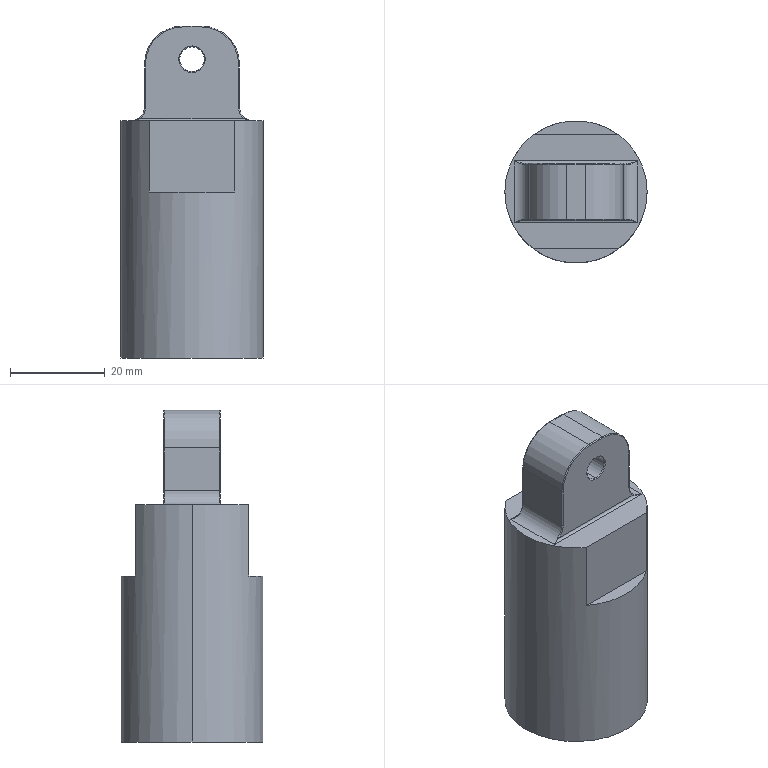Part | NX | features BREP 1 | 1 solid | 47 faces | box 30 x 30 x 70 mm | volume 29940 mm3 | cylinder 18 | plane 11 | torus 8 | cone 6 | spline 4 | commonest cylinder face diameters 0.4 x6 1 x2 5.2 x2 6 x2 16 x2 18.5 x2
STEP:
#1=CARTESIAN_POINT('',(0.,-5.8,65.6));
#2=VERTEX_POINT('',#1);
#3=CARTESIAN_POINT('',(0.,-5.8,60.4));
#4=VERTEX_POINT('',#3);
#5=CARTESIAN_POINT('',(0.,-5.8,63.));
#6=DIRECTION('',(0.,-1.,0.));
#7=DIRECTION('',(0.,0.,1.));
#8=AXIS2_PLACEMENT_3D('',#5,#6,#7);
#9=CIRCLE('',#8,2.6);
#10=EDGE_CURVE('',#2,#4,#9,.T.);
#11=ORIENTED_EDGE('',*,*,#10,.F.);
#12=CARTESIAN_POINT('',(0.,-6.,65.8));
#13=VERTEX_POINT('',#12);
#14=CARTESIAN_POINT('',(0.,-6.,65.8));
#15=DIRECTION('',(0.,-0.7071,0.7071));
#16=VECTOR('',#15,1000.);
#17=LINE('',#14,#16);
#18=EDGE_CURVE('',#2,#13,#17,.T.);
#19=ORIENTED_EDGE('',*,*,#18,.T.);
#20=CARTESIAN_POINT('',(0.,-6.,60.2));
#21=VERTEX_POINT('',#20);
#22=CARTESIAN_POINT('',(0.,-6.,63.));
#23=DIRECTION('',(0.,1.,0.));
#24=DIRECTION('',(-1.,0.,0.));
#25=AXIS2_PLACEMENT_3D('',#22,#23,#24);
#26=CIRCLE('',#25,2.8);
#27=EDGE_CURVE('',#21,#13,#26,.T.);
#28=ORIENTED_EDGE('',*,*,#27,.F.);
#29=CARTESIAN_POINT('',(0.,-6.,60.2));
#30=DIRECTION('',(0.,-0.7071,-0.7071));
#31=VECTOR('',#30,1000.);
#32=LINE('',#29,#31);
#33=EDGE_CURVE('',#4,#21,#32,.T.);
#34=ORIENTED_EDGE('',*,*,#33,.F.);
#35=EDGE_LOOP('',(#11,#19,#28,#34));
#36=FACE_BOUND('',#35,.T.);
#37=CARTESIAN_POINT('',(0.,-6.,63.));
#38=DIRECTION('',(0.,-1.,0.));
#39=DIRECTION('',(0.,0.,-1.));
#40=AXIS2_PLACEMENT_3D('',#37,#38,#39);
#41=CONICAL_SURFACE('',#40,2.8,0.7854);
#42=ADVANCED_FACE('',(#36),#41,.F.);
#43=CARTESIAN_POINT('',(0.,5.8,60.4));
#44=VERTEX_POINT('',#43);
#45=CARTESIAN_POINT('',(0.,5.8,65.6));
#46=VERTEX_POINT('',#45);
#47=CARTESIAN_POINT('',(0.,5.8,63.));
#48=DIRECTION('',(0.,1.,0.));
#49=DIRECTION('',(0.,0.,-1.));
#50=AXIS2_PLACEMENT_3D('',#47,#48,#49);
#51=CIRCLE('',#50,2.6);
#52=EDGE_CURVE('',#44,#46,#51,.T.);
#53=ORIENTED_EDGE('',*,*,#52,.F.);
#54=CARTESIAN_POINT('',(0.,6.,60.2));
#55=VERTEX_POINT('',#54);
#56=CARTESIAN_POINT('',(0.,5.8,60.4));
#57=DIRECTION('',(0.,0.7071,-0.7071));
#58=VECTOR('',#57,1000.);
#59=LINE('',#56,#58);
#60=EDGE_CURVE('',#55,#44,#59,.F.);
#61=ORIENTED_EDGE('',*,*,#60,.F.);
#62=CARTESIAN_POINT('',(0.,6.,65.8));
#63=VERTEX_POINT('',#62);
#64=CARTESIAN_POINT('',(0.,6.,63.));
#65=DIRECTION('',(0.,-1.,0.));
#66=DIRECTION('',(1.,0.,0.));
#67=AXIS2_PLACEMENT_3D('',#64,#65,#66);
#68=CIRCLE('',#67,2.8);
#69=EDGE_CURVE('',#63,#55,#68,.T.);
#70=ORIENTED_EDGE('',*,*,#69,.F.);
#71=CARTESIAN_POINT('',(0.,5.8,65.6));
#72=DIRECTION('',(0.,0.7071,0.7071));
#73=VECTOR('',#72,1000.);
#74=LINE('',#71,#73);
#75=EDGE_CURVE('',#63,#46,#74,.F.);
#76=ORIENTED_EDGE('',*,*,#75,.T.);
#77=EDGE_LOOP('',(#53,#61,#70,#76));
#78=FACE_BOUND('',#77,.T.);
#79=CARTESIAN_POINT('',(0.,5.8,63.));
#80=DIRECTION('',(0.,1.,0.));
#81=DIRECTION('',(0.,0.,1.));
#82=AXIS2_PLACEMENT_3D('',#79,#80,#81);
#83=CONICAL_SURFACE('',#82,2.6,0.7854);
#84=ADVANCED_FACE('',(#78),#83,.F.);
#85=ORIENTED_EDGE('',*,*,#10,.T.);
#86=CARTESIAN_POINT('',(0.,6.,60.4));
#87=DIRECTION('',(0.,1.,0.));
#88=VECTOR('',#87,1000.);
#89=LINE('',#86,#88);
#90=EDGE_CURVE('',#44,#4,#89,.F.);
#91=ORIENTED_EDGE('',*,*,#90,.F.);
#92=ORIENTED_EDGE('',*,*,#52,.T.);
#93=CARTESIAN_POINT('',(0.,6.,65.6));
#94=DIRECTION('',(0.,1.,0.));
#95=VECTOR('',#94,1000.);
#96=LINE('',#93,#95);
#97=EDGE_CURVE('',#46,#2,#96,.F.);
#98=ORIENTED_EDGE('',*,*,#97,.T.);
#99=EDGE_LOOP('',(#85,#91,#92,#98));
#100=FACE_BOUND('',#99,.T.);
#101=CARTESIAN_POINT('',(0.,6.,63.));
#102=DIRECTION('',(0.,1.,0.));
#103=DIRECTION('',(0.,0.,1.));
#104=AXIS2_PLACEMENT_3D('',#101,#102,#103);
#105=CYLINDRICAL_SURFACE('',#104,2.6);
#106=ADVANCED_FACE('',(#100),#105,.F.);
#107=CARTESIAN_POINT('',(9.25,0.,30.));
#108=VERTEX_POINT('',#107);
#109=CARTESIAN_POINT('',(-9.25,0.,30.));
#110=VERTEX_POINT('',#109);
#111=CARTESIAN_POINT('',(0.,0.,30.));
#112=DIRECTION('',(0.,0.,-1.));
#113=DIRECTION('',(-1.,0.,0.));
#114=AXIS2_PLACEMENT_3D('',#111,#112,#113);
#115=CIRCLE('',#114,9.25);
#116=EDGE_CURVE('',#108,#110,#115,.T.);
#117=ORIENTED_EDGE('',*,*,#116,.F.);
#118=CARTESIAN_POINT('',(9.25,0.,0.));
#119=VERTEX_POINT('',#118);
#120=CARTESIAN_POINT('',(9.25,0.,0.));
#121=DIRECTION('',(0.,0.,-1.));
#122=VECTOR('',#121,1000.);
#123=LINE('',#120,#122);
#124=EDGE_CURVE('',#108,#119,#123,.T.);
#125=ORIENTED_EDGE('',*,*,#124,.T.);
#126=CARTESIAN_POINT('',(-9.25,0.,0.));
#127=VERTEX_POINT('',#126);
#128=CARTESIAN_POINT('',(0.,0.,0.));
#129=DIRECTION('',(0.,0.,-1.));
#130=DIRECTION('',(-1.,0.,0.));
#131=AXIS2_PLACEMENT_3D('',#128,#129,#130);
#132=CIRCLE('',#131,9.25);
#133=EDGE_CURVE('',#119,#127,#132,.T.);
#134=ORIENTED_EDGE('',*,*,#133,.T.);
#135=CARTESIAN_POINT('',(-9.25,0.,0.));
#136=DIRECTION('',(0.,0.,-1.));
#137=VECTOR('',#136,1000.);
#138=LINE('',#135,#137);
#139=EDGE_CURVE('',#110,#127,#138,.T.);
#140=ORIENTED_EDGE('',*,*,#139,.F.);
#141=EDGE_LOOP('',(#117,#125,#134,#140));
#142=FACE_BOUND('',#141,.T.);
#143=CARTESIAN_POINT('',(0.,0.,0.));
#144=DIRECTION('',(0.,0.,-1.));
#145=DIRECTION('',(-1.,0.,0.));
#146=AXIS2_PLACEMENT_3D('',#143,#144,#145);
#147=CYLINDRICAL_SURFACE('',#146,9.25);
#148=ADVANCED_FACE('',(#142),#147,.F.);
#149=CARTESIAN_POINT('',(0.,0.,35.558));
#150=VERTEX_POINT('',#149);
#151=CARTESIAN_POINT('',(-9.25,0.,30.));
#152=DIRECTION('',(-0.8572,0.,-0.515));
#153=VECTOR('',#152,1000.);
#154=LINE('',#151,#153);
#155=EDGE_CURVE('',#150,#110,#154,.T.);
#156=ORIENTED_EDGE('',*,*,#155,.F.);
#157=CARTESIAN_POINT('',(9.25,0.,30.));
#158=DIRECTION('',(0.8572,0.,-0.515));
#159=VECTOR('',#158,1000.);
#160=LINE('',#157,#159);
#161=EDGE_CURVE('',#150,#108,#160,.T.);
#162=ORIENTED_EDGE('',*,*,#161,.T.);
#163=ORIENTED_EDGE('',*,*,#116,.T.);
#164=EDGE_LOOP('',(#156,#162,#163));
#165=FACE_BOUND('',#164,.T.);
#166=CARTESIAN_POINT('',(0.,0.,30.));
#167=DIRECTION('',(0.,0.,-1.));
#168=DIRECTION('',(-1.,0.,0.));
#169=AXIS2_PLACEMENT_3D('',#166,#167,#168);
#170=CONICAL_SURFACE('',#169,9.25,1.03);
#171=ADVANCED_FACE('',(#165),#170,.F.);
#172=CARTESIAN_POINT('',(15.,0.,50.));
#173=VERTEX_POINT('',#172);
#174=CARTESIAN_POINT('',(9.,12.,50.));
#175=VERTEX_POINT('',#174);
#176=CARTESIAN_POINT('',(0.,0.,50.));
#177=DIRECTION('',(0.,0.,1.));
#178=DIRECTION('',(1.,0.,0.));
#179=AXIS2_PLACEMENT_3D('',#176,#177,#178);
#180=CIRCLE('',#179,15.);
#181=EDGE_CURVE('',#173,#175,#180,.T.);
#182=ORIENTED_EDGE('',*,*,#181,.F.);
#183=CARTESIAN_POINT('',(15.,0.,0.));
#184=VERTEX_POINT('',#183);
#185=CARTESIAN_POINT('',(15.,0.,50.));
#186=DIRECTION('',(0.,0.,-1.));
#187=VECTOR('',#186,1000.);
#188=LINE('',#185,#187);
#189=EDGE_CURVE('',#173,#184,#188,.T.);
#190=ORIENTED_EDGE('',*,*,#189,.T.);
#191=CARTESIAN_POINT('',(-15.,0.,0.));
#192=VERTEX_POINT('',#191);
#193=CARTESIAN_POINT('',(0.,0.,0.));
#194=DIRECTION('',(0.,0.,1.));
#195=DIRECTION('',(1.,0.,0.));
#196=AXIS2_PLACEMENT_3D('',#193,#194,#195);
#197=CIRCLE('',#196,15.);
#198=EDGE_CURVE('',#184,#192,#197,.T.);
#199=ORIENTED_EDGE('',*,*,#198,.T.);
#200=CARTESIAN_POINT('',(-15.,0.,50.));
#201=VERTEX_POINT('',#200);
#202=CARTESIAN_POINT('',(-15.,0.,50.));
#203=DIRECTION('',(0.,0.,-1.));
#204=VECTOR('',#203,1000.);
#205=LINE('',#202,#204);
#206=EDGE_CURVE('',#201,#192,#205,.T.);
#207=ORIENTED_EDGE('',*,*,#206,.F.);
#208=CARTESIAN_POINT('',(-9.,12.,50.));
#209=VERTEX_POINT('',#208);
#210=CARTESIAN_POINT('',(0.,0.,50.));
#211=DIRECTION('',(0.,0.,1.));
#212=DIRECTION('',(1.,0.,0.));
#213=AXIS2_PLACEMENT_3D('',#210,#211,#212);
#214=CIRCLE('',#213,15.);
#215=EDGE_CURVE('',#209,#201,#214,.T.);
#216=ORIENTED_EDGE('',*,*,#215,.F.);
#217=CARTESIAN_POINT('',(-9.,12.,35.));
#218=VERTEX_POINT('',#217);
#219=CARTESIAN_POINT('',(-9.,12.,50.));
#220=DIRECTION('',(0.,0.,1.));
#221=VECTOR('',#220,1000.);
#222=LINE('',#219,#221);
#223=EDGE_CURVE('',#218,#209,#222,.T.);
#224=ORIENTED_EDGE('',*,*,#223,.F.);
#225=CARTESIAN_POINT('',(9.,12.,35.));
#226=VERTEX_POINT('',#225);
#227=CARTESIAN_POINT('',(0.,0.,35.));
#228=DIRECTION('',(0.,0.,1.));
#229=DIRECTION('',(1.,0.,0.));
#230=AXIS2_PLACEMENT_3D('',#227,#228,#229);
#231=CIRCLE('',#230,15.);
#232=EDGE_CURVE('',#226,#218,#231,.T.);
#233=ORIENTED_EDGE('',*,*,#232,.F.);
#234=CARTESIAN_POINT('',(9.,12.,50.));
#235=DIRECTION('',(0.,0.,-1.));
#236=VECTOR('',#235,1000.);
#237=LINE('',#234,#236);
#238=EDGE_CURVE('',#175,#226,#237,.T.);
#239=ORIENTED_EDGE('',*,*,#238,.F.);
#240=EDGE_LOOP('',(#182,#190,#199,#207,#216,#224,#233,#239));
#241=FACE_BOUND('',#240,.T.);
#242=CARTESIAN_POINT('',(0.,0.,50.));
#243=DIRECTION('',(0.,0.,-1.));
#244=DIRECTION('',(-1.,0.,0.));
#245=AXIS2_PLACEMENT_3D('',#242,#243,#244);
#246=CYLINDRICAL_SURFACE('',#245,15.);
#247=ADVANCED_FACE('',(#241),#246,.T.);
#248=ORIENTED_EDGE('',*,*,#189,.F.);
#249=CARTESIAN_POINT('',(9.,-12.,50.));
#250=VERTEX_POINT('',#249);
#251=CARTESIAN_POINT('',(0.,0.,50.));
#252=DIRECTION('',(0.,0.,1.));
#253=DIRECTION('',(1.,0.,0.));
#254=AXIS2_PLACEMENT_3D('',#251,#252,#253);
#255=CIRCLE('',#254,15.);
#256=EDGE_CURVE('',#250,#173,#255,.T.);
#257=ORIENTED_EDGE('',*,*,#256,.F.);
#258=CARTESIAN_POINT('',(9.,-12.,35.));
#259=VERTEX_POINT('',#258);
#260=CARTESIAN_POINT('',(9.,-12.,50.));
#261=DIRECTION('',(0.,0.,1.));
#262=VECTOR('',#261,1000.);
#263=LINE('',#260,#262);
#264=EDGE_CURVE('',#259,#250,#263,.T.);
#265=ORIENTED_EDGE('',*,*,#264,.F.);
#266=CARTESIAN_POINT('',(-9.,-12.,35.));
#267=VERTEX_POINT('',#266);
#268=CARTESIAN_POINT('',(0.,0.,35.));
#269=DIRECTION('',(0.,0.,1.));
#270=DIRECTION('',(1.,0.,0.));
#271=AXIS2_PLACEMENT_3D('',#268,#269,#270);
#272=CIRCLE('',#271,15.);
#273=EDGE_CURVE('',#267,#259,#272,.T.);
#274=ORIENTED_EDGE('',*,*,#273,.F.);
#275=CARTESIAN_POINT('',(-9.,-12.,50.));
#276=VERTEX_POINT('',#275);
#277=CARTESIAN_POINT('',(-9.,-12.,50.));
#278=DIRECTION('',(0.,0.,-1.));
#279=VECTOR('',#278,1000.);
#280=LINE('',#277,#279);
#281=EDGE_CURVE('',#276,#267,#280,.T.);
#282=ORIENTED_EDGE('',*,*,#281,.F.);
#283=CARTESIAN_POINT('',(0.,0.,50.));
#284=DIRECTION('',(0.,0.,1.));
#285=DIRECTION('',(1.,0.,0.));
#286=AXIS2_PLACEMENT_3D('',#283,#284,#285);
#287=CIRCLE('',#286,15.);
#288=EDGE_CURVE('',#201,#276,#287,.T.);
#289=ORIENTED_EDGE('',*,*,#288,.F.);
#290=ORIENTED_EDGE('',*,*,#206,.T.);
#291=CARTESIAN_POINT('',(0.,0.,0.));
#292=DIRECTION('',(0.,0.,1.));
#293=DIRECTION('',(1.,0.,0.));
#294=AXIS2_PLACEMENT_3D('',#291,#292,#293);
#295=CIRCLE('',#294,15.);
#296=EDGE_CURVE('',#192,#184,#295,.T.);
#297=ORIENTED_EDGE('',*,*,#296,.T.);
#298=EDGE_LOOP('',(#248,#257,#265,#274,#282,#289,#290,#297));
#299=FACE_BOUND('',#298,.T.);
#300=CARTESIAN_POINT('',(0.,0.,50.));
#301=DIRECTION('',(0.,0.,-1.));
#302=DIRECTION('',(-1.,0.,0.));
#303=AXIS2_PLACEMENT_3D('',#300,#301,#302);
#304=CYLINDRICAL_SURFACE('',#303,15.);
#305=ADVANCED_FACE('',(#299),#304,.T.);
#306=ORIENTED_EDGE('',*,*,#256,.T.);
#307=ORIENTED_EDGE('',*,*,#181,.T.);
#308=CARTESIAN_POINT('',(0.,12.,50.));
#309=DIRECTION('',(-1.,0.,0.));
#310=VECTOR('',#309,1000.);
#311=LINE('',#308,#310);
#312=EDGE_CURVE('',#175,#209,#311,.T.);
#313=ORIENTED_EDGE('',*,*,#312,.T.);
#314=ORIENTED_EDGE('',*,*,#215,.T.);
#315=ORIENTED_EDGE('',*,*,#288,.T.);
#316=CARTESIAN_POINT('',(0.,-12.,50.));
#317=DIRECTION('',(1.,0.,0.));
#318=VECTOR('',#317,1000.);
#319=LINE('',#316,#318);
#320=EDGE_CURVE('',#276,#250,#319,.T.);
#321=ORIENTED_EDGE('',*,*,#320,.T.);
#322=EDGE_LOOP('',(#306,#307,#313,#314,#315,#321));
#323=FACE_BOUND('',#322,.T.);
#324=CARTESIAN_POINT('',(13.,6.5,50.));
#325=VERTEX_POINT('',#324);
#326=CARTESIAN_POINT('',(13.,-6.5,50.));
#327=VERTEX_POINT('',#326);
#328=CARTESIAN_POINT('',(13.,0.,50.));
#329=DIRECTION('',(0.,-1.,0.));
#330=VECTOR('',#329,1000.);
#331=LINE('',#328,#330);
#332=EDGE_CURVE('',#325,#327,#331,.T.);
#333=ORIENTED_EDGE('',*,*,#332,.T.);
#334=CARTESIAN_POINT('',(-13.,-6.5,50.));
#335=VERTEX_POINT('',#334);
#336=CARTESIAN_POINT('',(0.,-6.5,50.));
#337=DIRECTION('',(-1.,0.,0.));
#338=VECTOR('',#337,1000.);
#339=LINE('',#336,#338);
#340=EDGE_CURVE('',#327,#335,#339,.T.);
#341=ORIENTED_EDGE('',*,*,#340,.T.);
#342=CARTESIAN_POINT('',(-13.,6.5,50.));
#343=VERTEX_POINT('',#342);
#344=CARTESIAN_POINT('',(-13.,0.,50.));
#345=DIRECTION('',(0.,1.,0.));
#346=VECTOR('',#345,1000.);
#347=LINE('',#344,#346);
#348=EDGE_CURVE('',#335,#343,#347,.T.);
#349=ORIENTED_EDGE('',*,*,#348,.T.);
#350=CARTESIAN_POINT('',(0.,6.5,50.));
#351=DIRECTION('',(1.,0.,0.));
#352=VECTOR('',#351,1000.);
#353=LINE('',#350,#352);
#354=EDGE_CURVE('',#343,#325,#353,.T.);
#355=ORIENTED_EDGE('',*,*,#354,.T.);
#356=EDGE_LOOP('',(#333,#341,#349,#355));
#357=FACE_BOUND('',#356,.T.);
#358=CARTESIAN_POINT('',(0.,0.,50.));
#359=DIRECTION('',(0.,0.,1.));
#360=DIRECTION('',(1.,0.,0.));
#361=AXIS2_PLACEMENT_3D('',#358,#359,#360);
#362=PLANE('',#361);
#363=ADVANCED_FACE('',(#323,#357),#362,.T.);
#364=ORIENTED_EDGE('',*,*,#296,.F.);
#365=ORIENTED_EDGE('',*,*,#198,.F.);
#366=EDGE_LOOP('',(#364,#365));
#367=FACE_BOUND('',#366,.T.);
#368=CARTESIAN_POINT('',(0.,0.,0.));
#369=DIRECTION('',(0.,0.,-1.));
#370=DIRECTION('',(-1.,0.,0.));
#371=AXIS2_PLACEMENT_3D('',#368,#369,#370);
#372=CIRCLE('',#371,9.25);
#373=EDGE_CURVE('',#127,#119,#372,.T.);
#374=ORIENTED_EDGE('',*,*,#373,.F.);
#375=ORIENTED_EDGE('',*,*,#133,.F.);
#376=EDGE_LOOP('',(#374,#375));
#377=FACE_BOUND('',#376,.T.);
#378=CARTESIAN_POINT('',(0.,0.,0.));
#379=DIRECTION('',(0.,0.,1.));
#380=DIRECTION('',(1.,0.,0.));
#381=AXIS2_PLACEMENT_3D('',#378,#379,#380);
#382=PLANE('',#381);
#383=ADVANCED_FACE('',(#367,#377),#382,.F.);
#384=ORIENTED_EDGE('',*,*,#161,.F.);
#385=ORIENTED_EDGE('',*,*,#155,.T.);
#386=CARTESIAN_POINT('',(0.,0.,30.));
#387=DIRECTION('',(0.,0.,-1.));
#388=DIRECTION('',(-1.,0.,0.));
#389=AXIS2_PLACEMENT_3D('',#386,#387,#388);
#390=CIRCLE('',#389,9.25);
#391=EDGE_CURVE('',#110,#108,#390,.T.);
#392=ORIENTED_EDGE('',*,*,#391,.T.);
#393=EDGE_LOOP('',(#384,#385,#392));
#394=FACE_BOUND('',#393,.T.);
#395=CARTESIAN_POINT('',(0.,0.,30.));
#396=DIRECTION('',(0.,0.,-1.));
#397=DIRECTION('',(-1.,0.,0.));
#398=AXIS2_PLACEMENT_3D('',#395,#396,#397);
#399=CONICAL_SURFACE('',#398,9.25,1.03);
#400=ADVANCED_FACE('',(#394),#399,.F.);
#401=ORIENTED_EDGE('',*,*,#124,.F.);
#402=ORIENTED_EDGE('',*,*,#391,.F.);
#403=ORIENTED_EDGE('',*,*,#139,.T.);
#404=ORIENTED_EDGE('',*,*,#373,.T.);
#405=EDGE_LOOP('',(#401,#402,#403,#404));
#406=FACE_BOUND('',#405,.T.);
#407=CARTESIAN_POINT('',(0.,0.,0.));
#408=DIRECTION('',(0.,0.,-1.));
#409=DIRECTION('',(-1.,0.,0.));
#410=AXIS2_PLACEMENT_3D('',#407,#408,#409);
#411=CYLINDRICAL_SURFACE('',#410,9.25);
#412=ADVANCED_FACE('',(#406),#411,.F.);
#413=CARTESIAN_POINT('',(-10.,5.8,53.));
#414=VERTEX_POINT('',#413);
#415=CARTESIAN_POINT('',(-10.,-5.8,53.));
#416=VERTEX_POINT('',#415);
#417=CARTESIAN_POINT('',(-10.,-6.,53.));
#418=DIRECTION('',(0.,-1.,0.));
#419=VECTOR('',#418,1000.);
#420=LINE('',#417,#419);
#421=EDGE_CURVE('',#414,#416,#420,.T.);
#422=ORIENTED_EDGE('',*,*,#421,.T.);
#423=CARTESIAN_POINT('',(-10.,-5.8,62.));
#424=VERTEX_POINT('',#423);
#425=CARTESIAN_POINT('',(-10.,-5.8,70.));
#426=DIRECTION('',(0.,0.,1.));
#427=VECTOR('',#426,1000.);
#428=LINE('',#425,#427);
#429=EDGE_CURVE('',#416,#424,#428,.T.);
#430=ORIENTED_EDGE('',*,*,#429,.T.);
#431=CARTESIAN_POINT('',(-10.,5.8,62.));
#432=VERTEX_POINT('',#431);
#433=CARTESIAN_POINT('',(-10.,6.,62.));
#434=DIRECTION('',(0.,1.,0.));
#435=VECTOR('',#434,1000.);
#436=LINE('',#433,#435);
#437=EDGE_CURVE('',#424,#432,#436,.T.);
#438=ORIENTED_EDGE('',*,*,#437,.T.);
#439=CARTESIAN_POINT('',(-10.,5.8,70.));
#440=DIRECTION('',(0.,0.,-1.));
#441=VECTOR('',#440,1000.);
#442=LINE('',#439,#441);
#443=EDGE_CURVE('',#432,#414,#442,.T.);
#444=ORIENTED_EDGE('',*,*,#443,.T.);
#445=EDGE_LOOP('',(#422,#430,#438,#444));
#446=FACE_BOUND('',#445,.T.);
#447=CARTESIAN_POINT('',(-10.,-6.,70.));
#448=DIRECTION('',(1.,0.,0.));
#449=DIRECTION('',(0.,1.,0.));
#450=AXIS2_PLACEMENT_3D('',#447,#448,#449);
#451=PLANE('',#450);
#452=ADVANCED_FACE('',(#446),#451,.F.);
#453=CARTESIAN_POINT('',(-11.003,-6.,50.5));
#454=VERTEX_POINT('',#453);
#455=CARTESIAN_POINT('',(11.003,-6.,50.5));
#456=VERTEX_POINT('',#455);
#457=CARTESIAN_POINT('',(10.,-6.,50.5));
#458=DIRECTION('',(1.,0.,0.));
#459=VECTOR('',#458,1000.);
#460=LINE('',#457,#459);
#461=EDGE_CURVE('',#454,#456,#460,.T.);
#462=ORIENTED_EDGE('',*,*,#461,.T.);
#463=CARTESIAN_POINT('',(9.8,-6.,53.));
#464=VERTEX_POINT('',#463);
#465=CARTESIAN_POINT('',(13.,-6.,53.));
#466=DIRECTION('',(0.,1.,0.));
#467=DIRECTION('',(-1.,0.,0.));
#468=AXIS2_PLACEMENT_3D('',#465,#466,#467);
#469=CIRCLE('',#468,3.2);
#470=EDGE_CURVE('',#456,#464,#469,.T.);
#471=ORIENTED_EDGE('',*,*,#470,.T.);
#472=CARTESIAN_POINT('',(9.8,-6.,62.));
#473=VERTEX_POINT('',#472);
#474=CARTESIAN_POINT('',(9.8,-6.,70.));
#475=DIRECTION('',(0.,0.,1.));
#476=VECTOR('',#475,1000.);
#477=LINE('',#474,#476);
#478=EDGE_CURVE('',#464,#473,#477,.T.);
#479=ORIENTED_EDGE('',*,*,#478,.T.);
#480=CARTESIAN_POINT('',(2.,-6.,69.8));
#481=VERTEX_POINT('',#480);
#482=CARTESIAN_POINT('',(2.,-6.,62.));
#483=DIRECTION('',(0.,-1.,0.));
#484=DIRECTION('',(-1.,0.,0.));
#485=AXIS2_PLACEMENT_3D('',#482,#483,#484);
#486=CIRCLE('',#485,7.8);
#487=EDGE_CURVE('',#473,#481,#486,.T.);
#488=ORIENTED_EDGE('',*,*,#487,.T.);
#489=CARTESIAN_POINT('',(-2.,-6.,69.8));
#490=VERTEX_POINT('',#489);
#491=CARTESIAN_POINT('',(-2.,-6.,69.8));
#492=DIRECTION('',(-1.,0.,0.));
#493=VECTOR('',#492,1000.);
#494=LINE('',#491,#493);
#495=EDGE_CURVE('',#481,#490,#494,.T.);
#496=ORIENTED_EDGE('',*,*,#495,.T.);
#497=CARTESIAN_POINT('',(-9.8,-6.,62.));
#498=VERTEX_POINT('',#497);
#499=CARTESIAN_POINT('',(-2.,-6.,62.));
#500=DIRECTION('',(0.,-1.,0.));
#501=DIRECTION('',(-1.,0.,0.));
#502=AXIS2_PLACEMENT_3D('',#499,#500,#501);
#503=CIRCLE('',#502,7.8);
#504=EDGE_CURVE('',#490,#498,#503,.T.);
#505=ORIENTED_EDGE('',*,*,#504,.T.);
#506=CARTESIAN_POINT('',(-9.8,-6.,53.));
#507=VERTEX_POINT('',#506);
#508=CARTESIAN_POINT('',(-9.8,-6.,70.));
#509=DIRECTION('',(0.,0.,-1.));
#510=VECTOR('',#509,1000.);
#511=LINE('',#508,#510);
#512=EDGE_CURVE('',#498,#507,#511,.T.);
#513=ORIENTED_EDGE('',*,*,#512,.T.);
#514=CARTESIAN_POINT('',(-13.,-6.,53.));
#515=DIRECTION('',(0.,1.,0.));
#516=DIRECTION('',(-1.,0.,0.));
#517=AXIS2_PLACEMENT_3D('',#514,#515,#516);
#518=CIRCLE('',#517,3.2);
#519=EDGE_CURVE('',#507,#454,#518,.T.);
#520=ORIENTED_EDGE('',*,*,#519,.T.);
#521=EDGE_LOOP('',(#462,#471,#479,#488,#496,#505,#513,#520));
#522=FACE_BOUND('',#521,.T.);
#523=ORIENTED_EDGE('',*,*,#27,.T.);
#524=CARTESIAN_POINT('',(0.,-6.,63.));
#525=DIRECTION('',(0.,1.,0.));
#526=DIRECTION('',(-1.,0.,0.));
#527=AXIS2_PLACEMENT_3D('',#524,#525,#526);
#528=CIRCLE('',#527,2.8);
#529=EDGE_CURVE('',#13,#21,#528,.T.);
#530=ORIENTED_EDGE('',*,*,#529,.T.);
#531=EDGE_LOOP('',(#523,#530));
#532=FACE_BOUND('',#531,.T.);
#533=CARTESIAN_POINT('',(10.,-6.,70.));
#534=DIRECTION('',(0.,1.,0.));
#535=DIRECTION('',(1.,0.,0.));
#536=AXIS2_PLACEMENT_3D('',#533,#534,#535);
#537=PLANE('',#536);
#538=ADVANCED_FACE('',(#522,#532),#537,.F.);
#539=CARTESIAN_POINT('',(10.,5.8,62.));
#540=VERTEX_POINT('',#539);
#541=CARTESIAN_POINT('',(10.,-5.8,62.));
#542=VERTEX_POINT('',#541);
#543=CARTESIAN_POINT('',(10.,-6.,62.));
#544=DIRECTION('',(0.,-1.,0.));
#545=VECTOR('',#544,1000.);
#546=LINE('',#543,#545);
#547=EDGE_CURVE('',#540,#542,#546,.T.);
#548=ORIENTED_EDGE('',*,*,#547,.T.);
#549=CARTESIAN_POINT('',(10.,-5.8,53.));
#550=VERTEX_POINT('',#549);
#551=CARTESIAN_POINT('',(10.,-5.8,70.));
#552=DIRECTION('',(0.,0.,-1.));
#553=VECTOR('',#552,1000.);
#554=LINE('',#551,#553);
#555=EDGE_CURVE('',#542,#550,#554,.T.);
#556=ORIENTED_EDGE('',*,*,#555,.T.);
#557=CARTESIAN_POINT('',(10.,5.8,53.));
#558=VERTEX_POINT('',#557);
#559=CARTESIAN_POINT('',(10.,-6.,53.));
#560=DIRECTION('',(0.,1.,0.));
#561=VECTOR('',#560,1000.);
#562=LINE('',#559,#561);
#563=EDGE_CURVE('',#550,#558,#562,.T.);
#564=ORIENTED_EDGE('',*,*,#563,.T.);
#565=CARTESIAN_POINT('',(10.,5.8,70.));
#566=DIRECTION('',(0.,0.,1.));
#567=VECTOR('',#566,1000.);
#568=LINE('',#565,#567);
#569=EDGE_CURVE('',#558,#540,#568,.T.);
#570=ORIENTED_EDGE('',*,*,#569,.T.);
#571=EDGE_LOOP('',(#548,#556,#564,#570));
#572=FACE_BOUND('',#571,.T.);
#573=CARTESIAN_POINT('',(10.,-6.,70.));
#574=DIRECTION('',(-1.,0.,0.));
#575=DIRECTION('',(0.,0.,1.));
#576=AXIS2_PLACEMENT_3D('',#573,#574,#575);
#577=PLANE('',#576);
#578=ADVANCED_FACE('',(#572),#577,.F.);
#579=CARTESIAN_POINT('',(9.8,6.,62.));
#580=VERTEX_POINT('',#579);
#581=CARTESIAN_POINT('',(9.8,6.,53.));
#582=VERTEX_POINT('',#581);
#583=CARTESIAN_POINT('',(9.8,6.,70.));
#584=DIRECTION('',(0.,0.,-1.));
#585=VECTOR('',#584,1000.);
#586=LINE('',#583,#585);
#587=EDGE_CURVE('',#580,#582,#586,.T.);
#588=ORIENTED_EDGE('',*,*,#587,.T.);
#589=CARTESIAN_POINT('',(11.003,6.,50.5));
#590=VERTEX_POINT('',#589);
#591=CARTESIAN_POINT('',(13.,6.,53.));
#592=DIRECTION('',(0.,-1.,0.));
#593=DIRECTION('',(1.,0.,0.));
#594=AXIS2_PLACEMENT_3D('',#591,#592,#593);
#595=CIRCLE('',#594,3.2);
#596=EDGE_CURVE('',#582,#590,#595,.T.);
#597=ORIENTED_EDGE('',*,*,#596,.T.);
#598=CARTESIAN_POINT('',(-11.003,6.,50.5));
#599=VERTEX_POINT('',#598);
#600=CARTESIAN_POINT('',(10.,6.,50.5));
#601=DIRECTION('',(-1.,0.,0.));
#602=VECTOR('',#601,1000.);
#603=LINE('',#600,#602);
#604=EDGE_CURVE('',#590,#599,#603,.T.);
#605=ORIENTED_EDGE('',*,*,#604,.T.);
#606=CARTESIAN_POINT('',(-9.8,6.,53.));
#607=VERTEX_POINT('',#606);
#608=CARTESIAN_POINT('',(-13.,6.,53.));
#609=DIRECTION('',(0.,-1.,0.));
#610=DIRECTION('',(1.,0.,0.));
#611=AXIS2_PLACEMENT_3D('',#608,#609,#610);
#612=CIRCLE('',#611,3.2);
#613=EDGE_CURVE('',#599,#607,#612,.T.);
#614=ORIENTED_EDGE('',*,*,#613,.T.);
#615=CARTESIAN_POINT('',(-9.8,6.,62.));
#616=VERTEX_POINT('',#615);
#617=CARTESIAN_POINT('',(-9.8,6.,70.));
#618=DIRECTION('',(0.,0.,1.));
#619=VECTOR('',#618,1000.);
#620=LINE('',#617,#619);
#621=EDGE_CURVE('',#607,#616,#620,.T.);
#622=ORIENTED_EDGE('',*,*,#621,.T.);
#623=CARTESIAN_POINT('',(-2.,6.,69.8));
#624=VERTEX_POINT('',#623);
#625=CARTESIAN_POINT('',(-2.,6.,62.));
#626=DIRECTION('',(0.,1.,0.));
#627=DIRECTION('',(1.,0.,0.));
#628=AXIS2_PLACEMENT_3D('',#625,#626,#627);
#629=CIRCLE('',#628,7.8);
#630=EDGE_CURVE('',#616,#624,#629,.T.);
#631=ORIENTED_EDGE('',*,*,#630,.T.);
#632=CARTESIAN_POINT('',(2.,6.,69.8));
#633=VERTEX_POINT('',#632);
#634=CARTESIAN_POINT('',(2.,6.,69.8));
#635=DIRECTION('',(1.,0.,0.));
#636=VECTOR('',#635,1000.);
#637=LINE('',#634,#636);
#638=EDGE_CURVE('',#624,#633,#637,.T.);
#639=ORIENTED_EDGE('',*,*,#638,.T.);
#640=CARTESIAN_POINT('',(2.,6.,62.));
#641=DIRECTION('',(0.,1.,0.));
#642=DIRECTION('',(1.,0.,0.));
#643=AXIS2_PLACEMENT_3D('',#640,#641,#642);
#644=CIRCLE('',#643,7.8);
#645=EDGE_CURVE('',#633,#580,#644,.T.);
#646=ORIENTED_EDGE('',*,*,#645,.T.);
#647=EDGE_LOOP('',(#588,#597,#605,#614,#622,#631,#639,#646));
#648=FACE_BOUND('',#647,.T.);
#649=ORIENTED_EDGE('',*,*,#69,.T.);
#650=CARTESIAN_POINT('',(0.,6.,63.));
#651=DIRECTION('',(0.,-1.,0.));
#652=DIRECTION('',(1.,0.,0.));
#653=AXIS2_PLACEMENT_3D('',#650,#651,#652);
#654=CIRCLE('',#653,2.8);
#655=EDGE_CURVE('',#55,#63,#654,.T.);
#656=ORIENTED_EDGE('',*,*,#655,.T.);
#657=EDGE_LOOP('',(#649,#656));
#658=FACE_BOUND('',#657,.T.);
#659=CARTESIAN_POINT('',(10.,6.,70.));
#660=DIRECTION('',(0.,-1.,0.));
#661=DIRECTION('',(0.,0.,-1.));
#662=AXIS2_PLACEMENT_3D('',#659,#660,#661);
#663=PLANE('',#662);
#664=ADVANCED_FACE('',(#648,#658),#663,.F.);
#665=CARTESIAN_POINT('',(-2.,5.8,70.));
#666=VERTEX_POINT('',#665);
#667=CARTESIAN_POINT('',(-2.,-5.8,70.));
#668=VERTEX_POINT('',#667);
#669=CARTESIAN_POINT('',(-2.,-6.,70.));
#670=DIRECTION('',(0.,-1.,0.));
#671=VECTOR('',#670,1000.);
#672=LINE('',#669,#671);
#673=EDGE_CURVE('',#666,#668,#672,.T.);
#674=ORIENTED_EDGE('',*,*,#673,.T.);
#675=CARTESIAN_POINT('',(2.,-5.8,70.));
#676=VERTEX_POINT('',#675);
#677=CARTESIAN_POINT('',(2.,-5.8,70.));
#678=DIRECTION('',(1.,0.,0.));
#679=VECTOR('',#678,1000.);
#680=LINE('',#677,#679);
#681=EDGE_CURVE('',#668,#676,#680,.T.);
#682=ORIENTED_EDGE('',*,*,#681,.T.);
#683=CARTESIAN_POINT('',(2.,5.8,70.));
#684=VERTEX_POINT('',#683);
#685=CARTESIAN_POINT('',(2.,6.,70.));
#686=DIRECTION('',(0.,1.,0.));
#687=VECTOR('',#686,1000.);
#688=LINE('',#685,#687);
#689=EDGE_CURVE('',#676,#684,#688,.T.);
#690=ORIENTED_EDGE('',*,*,#689,.T.);
#691=CARTESIAN_POINT('',(-2.,5.8,70.));
#692=DIRECTION('',(-1.,0.,0.));
#693=VECTOR('',#692,1000.);
#694=LINE('',#691,#693);
#695=EDGE_CURVE('',#684,#666,#694,.T.);
#696=ORIENTED_EDGE('',*,*,#695,.T.);
#697=EDGE_LOOP('',(#674,#682,#690,#696));
#698=FACE_BOUND('',#697,.T.);
#699=CARTESIAN_POINT('',(0.,0.,70.));
#700=DIRECTION('',(0.,0.,1.));
#701=DIRECTION('',(1.,0.,0.));
#702=AXIS2_PLACEMENT_3D('',#699,#700,#701);
#703=PLANE('',#702);
#704=ADVANCED_FACE('',(#698),#703,.T.);
#705=ORIENTED_EDGE('',*,*,#90,.T.);
#706=CARTESIAN_POINT('',(0.,-5.8,63.));
#707=DIRECTION('',(0.,-1.,0.));
#708=DIRECTION('',(0.,0.,1.));
#709=AXIS2_PLACEMENT_3D('',#706,#707,#708);
#710=CIRCLE('',#709,2.6);
#711=EDGE_CURVE('',#4,#2,#710,.T.);
#712=ORIENTED_EDGE('',*,*,#711,.T.);
#713=ORIENTED_EDGE('',*,*,#97,.F.);
#714=CARTESIAN_POINT('',(0.,5.8,63.));
#715=DIRECTION('',(0.,1.,0.));
#716=DIRECTION('',(0.,0.,-1.));
#717=AXIS2_PLACEMENT_3D('',#714,#715,#716);
#718=CIRCLE('',#717,2.6);
#719=EDGE_CURVE('',#46,#44,#718,.T.);
#720=ORIENTED_EDGE('',*,*,#719,.T.);
#721=EDGE_LOOP('',(#705,#712,#713,#720));
#722=FACE_BOUND('',#721,.T.);
#723=CARTESIAN_POINT('',(0.,6.,63.));
#724=DIRECTION('',(0.,1.,0.));
#725=DIRECTION('',(0.,0.,1.));
#726=AXIS2_PLACEMENT_3D('',#723,#724,#725);
#727=CYLINDRICAL_SURFACE('',#726,2.6);
#728=ADVANCED_FACE('',(#722),#727,.F.);
#729=CARTESIAN_POINT('',(11.127,-5.8,50.656));
#730=VERTEX_POINT('',#729);
#731=CARTESIAN_POINT('',(13.,-5.8,53.));
#732=DIRECTION('',(0.,-1.,0.));
#733=DIRECTION('',(-1.,0.,0.));
#734=AXIS2_PLACEMENT_3D('',#731,#732,#733);
#735=CIRCLE('',#734,3.);
#736=EDGE_CURVE('',#550,#730,#735,.T.);
#737=ORIENTED_EDGE('',*,*,#736,.T.);
#738=CARTESIAN_POINT('',(11.127,-5.8,50.656));
#739=CARTESIAN_POINT('',(11.24,-5.8,50.567));
#740=CARTESIAN_POINT('',(11.481,-5.832,50.389));
#741=CARTESIAN_POINT('',(11.986,-6.018,50.169));
#742=CARTESIAN_POINT('',(12.246,-6.134,50.093));
#743=CARTESIAN_POINT('',(12.543,-6.273,50.032));
#744=CARTESIAN_POINT('',(12.687,-6.345,50.014));
#745=CARTESIAN_POINT('',(12.89,-6.445,50.));
#746=CARTESIAN_POINT('',(13.,-6.5,50.));
#747=B_SPLINE_CURVE_WITH_KNOTS('',3,(#738,#739,#740,#741,#742,#743,#744,#745,#746),.UNSPECIFIED.,.F.,.F.,(4,1,1,1,1,1,4),(0.,0.25,0.5,0.625,0.75,0.875,1.),.UNSPECIFIED.);
#748=EDGE_CURVE('',#730,#327,#747,.T.);
#749=ORIENTED_EDGE('',*,*,#748,.T.);
#750=ORIENTED_EDGE('',*,*,#332,.F.);
#751=CARTESIAN_POINT('',(11.127,5.8,50.656));
#752=VERTEX_POINT('',#751);
#753=CARTESIAN_POINT('',(13.,6.5,50.));
#754=CARTESIAN_POINT('',(12.889,6.445,50.));
#755=CARTESIAN_POINT('',(12.687,6.345,50.014));
#756=CARTESIAN_POINT('',(12.542,6.273,50.032));
#757=CARTESIAN_POINT('',(12.248,6.134,50.092));
#758=CARTESIAN_POINT('',(11.84,5.955,50.213));
#759=CARTESIAN_POINT('',(11.379,5.8,50.455));
#760=CARTESIAN_POINT('',(11.127,5.8,50.656));
#761=B_SPLINE_CURVE_WITH_KNOTS('',3,(#753,#754,#755,#756,#757,#758,#759,#760),.UNSPECIFIED.,.F.,.F.,(4,1,1,1,1,4),(0.,0.125,0.25,0.375,0.5,1.),.UNSPECIFIED.);
#762=EDGE_CURVE('',#325,#752,#761,.T.);
#763=ORIENTED_EDGE('',*,*,#762,.T.);
#764=CARTESIAN_POINT('',(13.,5.8,53.));
#765=DIRECTION('',(0.,1.,0.));
#766=DIRECTION('',(1.,0.,0.));
#767=AXIS2_PLACEMENT_3D('',#764,#765,#766);
#768=CIRCLE('',#767,3.);
#769=EDGE_CURVE('',#752,#558,#768,.T.);
#770=ORIENTED_EDGE('',*,*,#769,.T.);
#771=ORIENTED_EDGE('',*,*,#563,.F.);
#772=EDGE_LOOP('',(#737,#749,#750,#763,#770,#771));
#773=FACE_BOUND('',#772,.T.);
#774=CARTESIAN_POINT('',(13.,-6.,53.));
#775=DIRECTION('',(0.,1.,0.));
#776=DIRECTION('',(0.,0.,1.));
#777=AXIS2_PLACEMENT_3D('',#774,#775,#776);
#778=CYLINDRICAL_SURFACE('',#777,3.);
#779=ADVANCED_FACE('',(#773),#778,.F.);
#780=ORIENTED_EDGE('',*,*,#348,.F.);
#781=CARTESIAN_POINT('',(-11.127,-5.8,50.656));
#782=VERTEX_POINT('',#781);
#783=CARTESIAN_POINT('',(-13.,-6.5,50.));
#784=CARTESIAN_POINT('',(-12.889,-6.445,50.));
#785=CARTESIAN_POINT('',(-12.687,-6.345,50.014));
#786=CARTESIAN_POINT('',(-12.542,-6.273,50.032));
#787=CARTESIAN_POINT('',(-12.248,-6.134,50.092));
#788=CARTESIAN_POINT('',(-11.84,-5.955,50.213));
#789=CARTESIAN_POINT('',(-11.379,-5.8,50.455));
#790=CARTESIAN_POINT('',(-11.127,-5.8,50.656));
#791=B_SPLINE_CURVE_WITH_KNOTS('',3,(#783,#784,#785,#786,#787,#788,#789,#790),.UNSPECIFIED.,.F.,.F.,(4,1,1,1,1,4),(0.,0.125,0.25,0.375,0.5,1.),.UNSPECIFIED.);
#792=EDGE_CURVE('',#335,#782,#791,.T.);
#793=ORIENTED_EDGE('',*,*,#792,.T.);
#794=CARTESIAN_POINT('',(-13.,-5.8,53.));
#795=DIRECTION('',(0.,-1.,0.));
#796=DIRECTION('',(-1.,0.,0.));
#797=AXIS2_PLACEMENT_3D('',#794,#795,#796);
#798=CIRCLE('',#797,3.);
#799=EDGE_CURVE('',#782,#416,#798,.T.);
#800=ORIENTED_EDGE('',*,*,#799,.T.);
#801=ORIENTED_EDGE('',*,*,#421,.F.);
#802=CARTESIAN_POINT('',(-11.127,5.8,50.656));
#803=VERTEX_POINT('',#802);
#804=CARTESIAN_POINT('',(-13.,5.8,53.));
#805=DIRECTION('',(0.,1.,0.));
#806=DIRECTION('',(1.,0.,0.));
#807=AXIS2_PLACEMENT_3D('',#804,#805,#806);
#808=CIRCLE('',#807,3.);
#809=EDGE_CURVE('',#414,#803,#808,.T.);
#810=ORIENTED_EDGE('',*,*,#809,.T.);
#811=CARTESIAN_POINT('',(-11.127,5.8,50.656));
#812=CARTESIAN_POINT('',(-11.24,5.8,50.567));
#813=CARTESIAN_POINT('',(-11.481,5.832,50.389));
#814=CARTESIAN_POINT('',(-11.986,6.018,50.169));
#815=CARTESIAN_POINT('',(-12.246,6.134,50.093));
#816=CARTESIAN_POINT('',(-12.543,6.273,50.032));
#817=CARTESIAN_POINT('',(-12.687,6.345,50.014));
#818=CARTESIAN_POINT('',(-12.89,6.445,50.));
#819=CARTESIAN_POINT('',(-13.,6.5,50.));
#820=B_SPLINE_CURVE_WITH_KNOTS('',3,(#811,#812,#813,#814,#815,#816,#817,#818,#819),.UNSPECIFIED.,.F.,.F.,(4,1,1,1,1,1,4),(0.,0.25,0.5,0.625,0.75,0.875,1.),.UNSPECIFIED.);
#821=EDGE_CURVE('',#803,#343,#820,.T.);
#822=ORIENTED_EDGE('',*,*,#821,.T.);
#823=EDGE_LOOP('',(#780,#793,#800,#801,#810,#822));
#824=FACE_BOUND('',#823,.T.);
#825=CARTESIAN_POINT('',(-13.,-6.,53.));
#826=DIRECTION('',(0.,-1.,0.));
#827=DIRECTION('',(0.,0.,-1.));
#828=AXIS2_PLACEMENT_3D('',#825,#826,#827);
#829=CYLINDRICAL_SURFACE('',#828,3.);
#830=ADVANCED_FACE('',(#824),#829,.F.);
#831=ORIENTED_EDGE('',*,*,#340,.F.);
#832=CARTESIAN_POINT('',(13.,-6.5,50.));
#833=CARTESIAN_POINT('',(12.769,-6.423,50.));
#834=CARTESIAN_POINT('',(12.475,-6.324,50.025));
#835=CARTESIAN_POINT('',(12.148,-6.225,50.082));
#836=CARTESIAN_POINT('',(12.021,-6.187,50.107));
#837=CARTESIAN_POINT('',(11.67,-6.092,50.202));
#838=CARTESIAN_POINT('',(11.338,-6.023,50.326));
#839=CARTESIAN_POINT('',(11.12,-6.,50.433));
#840=CARTESIAN_POINT('',(11.003,-6.,50.5));
#841=B_SPLINE_CURVE_WITH_KNOTS('',3,(#832,#833,#834,#835,#836,#837,#838,#839,#840),.UNSPECIFIED.,.F.,.F.,(4,1,1,1,1,1,4),(0.,0.25,0.375,0.5,0.625,0.75,1.),.UNSPECIFIED.);
#842=EDGE_CURVE('',#327,#456,#841,.T.);
#843=ORIENTED_EDGE('',*,*,#842,.T.);
#844=ORIENTED_EDGE('',*,*,#461,.F.);
#845=CARTESIAN_POINT('',(-11.003,-6.,50.5));
#846=CARTESIAN_POINT('',(-11.12,-6.,50.433));
#847=CARTESIAN_POINT('',(-11.338,-6.023,50.326));
#848=CARTESIAN_POINT('',(-11.67,-6.092,50.202));
#849=CARTESIAN_POINT('',(-12.021,-6.187,50.107));
#850=CARTESIAN_POINT('',(-12.148,-6.225,50.082));
#851=CARTESIAN_POINT('',(-12.475,-6.324,50.025));
#852=CARTESIAN_POINT('',(-12.768,-6.423,50.));
#853=CARTESIAN_POINT('',(-13.,-6.5,50.));
#854=B_SPLINE_CURVE_WITH_KNOTS('',3,(#845,#846,#847,#848,#849,#850,#851,#852,#853),.UNSPECIFIED.,.F.,.F.,(4,1,1,1,1,1,4),(0.,0.25,0.375,0.5,0.625,0.75,1.),.UNSPECIFIED.);
#855=EDGE_CURVE('',#454,#335,#854,.T.);
#856=ORIENTED_EDGE('',*,*,#855,.T.);
#857=EDGE_LOOP('',(#831,#843,#844,#856));
#858=FACE_BOUND('',#857,.T.);
#859=CARTESIAN_POINT('',(10.,-6.5,50.5));
#860=DIRECTION('',(1.,0.,0.));
#861=DIRECTION('',(0.,1.,0.));
#862=AXIS2_PLACEMENT_3D('',#859,#860,#861);
#863=CYLINDRICAL_SURFACE('',#862,0.5);
#864=ADVANCED_FACE('',(#858),#863,.F.);
#865=ORIENTED_EDGE('',*,*,#604,.F.);
#866=CARTESIAN_POINT('',(11.003,6.,50.5));
#867=CARTESIAN_POINT('',(11.12,6.,50.433));
#868=CARTESIAN_POINT('',(11.338,6.023,50.326));
#869=CARTESIAN_POINT('',(11.67,6.092,50.202));
#870=CARTESIAN_POINT('',(12.021,6.187,50.107));
#871=CARTESIAN_POINT('',(12.148,6.225,50.082));
#872=CARTESIAN_POINT('',(12.475,6.324,50.025));
#873=CARTESIAN_POINT('',(12.768,6.423,50.));
#874=CARTESIAN_POINT('',(13.,6.5,50.));
#875=B_SPLINE_CURVE_WITH_KNOTS('',3,(#866,#867,#868,#869,#870,#871,#872,#873,#874),.UNSPECIFIED.,.F.,.F.,(4,1,1,1,1,1,4),(0.,0.25,0.375,0.5,0.625,0.75,1.),.UNSPECIFIED.);
#876=EDGE_CURVE('',#590,#325,#875,.T.);
#877=ORIENTED_EDGE('',*,*,#876,.T.);
#878=ORIENTED_EDGE('',*,*,#354,.F.);
#879=CARTESIAN_POINT('',(-13.,6.5,50.));
#880=CARTESIAN_POINT('',(-12.769,6.423,50.));
#881=CARTESIAN_POINT('',(-12.475,6.324,50.025));
#882=CARTESIAN_POINT('',(-12.148,6.225,50.082));
#883=CARTESIAN_POINT('',(-12.021,6.187,50.107));
#884=CARTESIAN_POINT('',(-11.67,6.092,50.202));
#885=CARTESIAN_POINT('',(-11.338,6.023,50.326));
#886=CARTESIAN_POINT('',(-11.12,6.,50.433));
#887=CARTESIAN_POINT('',(-11.003,6.,50.5));
#888=B_SPLINE_CURVE_WITH_KNOTS('',3,(#879,#880,#881,#882,#883,#884,#885,#886,#887),.UNSPECIFIED.,.F.,.F.,(4,1,1,1,1,1,4),(0.,0.25,0.375,0.5,0.625,0.75,1.),.UNSPECIFIED.);
#889=EDGE_CURVE('',#343,#599,#888,.T.);
#890=ORIENTED_EDGE('',*,*,#889,.T.);
#891=EDGE_LOOP('',(#865,#877,#878,#890));
#892=FACE_BOUND('',#891,.T.);
#893=CARTESIAN_POINT('',(10.,6.5,50.5));
#894=DIRECTION('',(-1.,0.,0.));
#895=DIRECTION('',(0.,-1.,0.));
#896=AXIS2_PLACEMENT_3D('',#893,#894,#895);
#897=CYLINDRICAL_SURFACE('',#896,0.5);
#898=ADVANCED_FACE('',(#892),#897,.F.);
#899=ORIENTED_EDGE('',*,*,#281,.T.);
#900=CARTESIAN_POINT('',(25.302,-12.,35.));
#901=DIRECTION('',(1.,0.,0.));
#902=VECTOR('',#901,1000.);
#903=LINE('',#900,#902);
#904=EDGE_CURVE('',#267,#259,#903,.T.);
#905=ORIENTED_EDGE('',*,*,#904,.T.);
#906=ORIENTED_EDGE('',*,*,#264,.T.);
#907=ORIENTED_EDGE('',*,*,#320,.F.);
#908=EDGE_LOOP('',(#899,#905,#906,#907));
#909=FACE_BOUND('',#908,.T.);
#910=CARTESIAN_POINT('',(25.302,-12.,35.));
#911=DIRECTION('',(0.,-1.,0.));
#912=DIRECTION('',(0.,0.,-1.));
#913=AXIS2_PLACEMENT_3D('',#910,#911,#912);
#914=PLANE('',#913);
#915=ADVANCED_FACE('',(#909),#914,.T.);
#916=ORIENTED_EDGE('',*,*,#273,.T.);
#917=ORIENTED_EDGE('',*,*,#904,.F.);
#918=EDGE_LOOP('',(#916,#917));
#919=FACE_BOUND('',#918,.T.);
#920=CARTESIAN_POINT('',(0.,0.,35.));
#921=DIRECTION('',(0.,0.,1.));
#922=DIRECTION('',(1.,0.,0.));
#923=AXIS2_PLACEMENT_3D('',#920,#921,#922);
#924=PLANE('',#923);
#925=ADVANCED_FACE('',(#919),#924,.T.);
#926=ORIENTED_EDGE('',*,*,#232,.T.);
#927=CARTESIAN_POINT('',(25.302,12.,35.));
#928=DIRECTION('',(-1.,0.,0.));
#929=VECTOR('',#928,1000.);
#930=LINE('',#927,#929);
#931=EDGE_CURVE('',#226,#218,#930,.T.);
#932=ORIENTED_EDGE('',*,*,#931,.F.);
#933=EDGE_LOOP('',(#926,#932));
#934=FACE_BOUND('',#933,.T.);
#935=CARTESIAN_POINT('',(0.,0.,35.));
#936=DIRECTION('',(0.,0.,1.));
#937=DIRECTION('',(1.,0.,0.));
#938=AXIS2_PLACEMENT_3D('',#935,#936,#937);
#939=PLANE('',#938);
#940=ADVANCED_FACE('',(#934),#939,.T.);
#941=ORIENTED_EDGE('',*,*,#238,.T.);
#942=ORIENTED_EDGE('',*,*,#931,.T.);
#943=ORIENTED_EDGE('',*,*,#223,.T.);
#944=ORIENTED_EDGE('',*,*,#312,.F.);
#945=EDGE_LOOP('',(#941,#942,#943,#944));
#946=FACE_BOUND('',#945,.T.);
#947=CARTESIAN_POINT('',(25.302,12.,35.));
#948=DIRECTION('',(0.,1.,0.));
#949=DIRECTION('',(1.,0.,0.));
#950=AXIS2_PLACEMENT_3D('',#947,#948,#949);
#951=PLANE('',#950);
#952=ADVANCED_FACE('',(#946),#951,.T.);
#953=ORIENTED_EDGE('',*,*,#689,.F.);
#954=CARTESIAN_POINT('',(2.,-5.8,62.));
#955=DIRECTION('',(0.,1.,0.));
#956=DIRECTION('',(-1.,0.,0.));
#957=AXIS2_PLACEMENT_3D('',#954,#955,#956);
#958=CIRCLE('',#957,8.);
#959=EDGE_CURVE('',#676,#542,#958,.T.);
#960=ORIENTED_EDGE('',*,*,#959,.T.);
#961=ORIENTED_EDGE('',*,*,#547,.F.);
#962=CARTESIAN_POINT('',(2.,5.8,62.));
#963=DIRECTION('',(0.,-1.,0.));
#964=DIRECTION('',(1.,0.,0.));
#965=AXIS2_PLACEMENT_3D('',#962,#963,#964);
#966=CIRCLE('',#965,8.);
#967=EDGE_CURVE('',#540,#684,#966,.T.);
#968=ORIENTED_EDGE('',*,*,#967,.T.);
#969=EDGE_LOOP('',(#953,#960,#961,#968));
#970=FACE_BOUND('',#969,.T.);
#971=CARTESIAN_POINT('',(2.,0.,62.));
#972=DIRECTION('',(0.,-1.,0.));
#973=DIRECTION('',(0.,0.,-1.));
#974=AXIS2_PLACEMENT_3D('',#971,#972,#973);
#975=CYLINDRICAL_SURFACE('',#974,8.);
#976=ADVANCED_FACE('',(#970),#975,.T.);
#977=ORIENTED_EDGE('',*,*,#673,.F.);
#978=CARTESIAN_POINT('',(-2.,5.8,62.));
#979=DIRECTION('',(0.,-1.,0.));
#980=DIRECTION('',(1.,0.,0.));
#981=AXIS2_PLACEMENT_3D('',#978,#979,#980);
#982=CIRCLE('',#981,8.);
#983=EDGE_CURVE('',#666,#432,#982,.T.);
#984=ORIENTED_EDGE('',*,*,#983,.T.);
#985=ORIENTED_EDGE('',*,*,#437,.F.);
#986=CARTESIAN_POINT('',(-2.,-5.8,62.));
#987=DIRECTION('',(0.,1.,0.));
#988=DIRECTION('',(-1.,0.,0.));
#989=AXIS2_PLACEMENT_3D('',#986,#987,#988);
#990=CIRCLE('',#989,8.);
#991=EDGE_CURVE('',#424,#668,#990,.T.);
#992=ORIENTED_EDGE('',*,*,#991,.T.);
#993=EDGE_LOOP('',(#977,#984,#985,#992));
#994=FACE_BOUND('',#993,.T.);
#995=CARTESIAN_POINT('',(-2.,0.,62.));
#996=DIRECTION('',(0.,1.,0.));
#997=DIRECTION('',(0.,0.,1.));
#998=AXIS2_PLACEMENT_3D('',#995,#996,#997);
#999=CYLINDRICAL_SURFACE('',#998,8.);
#1000=ADVANCED_FACE('',(#994),#999,.T.);
#1001=ORIENTED_EDGE('',*,*,#792,.F.);
#1002=ORIENTED_EDGE('',*,*,#855,.F.);
#1003=CARTESIAN_POINT('',(-11.003,-5.8,50.5));
#1004=DIRECTION('',(0.7812,0.,0.6242));
#1005=DIRECTION('',(0.6242,0.,-0.7812));
#1006=AXIS2_PLACEMENT_3D('',#1003,#1004,#1005);
#1007=CIRCLE('',#1006,0.2);
#1008=EDGE_CURVE('',#782,#454,#1007,.T.);
#1009=ORIENTED_EDGE('',*,*,#1008,.F.);
#1010=EDGE_LOOP('',(#1001,#1002,#1009));
#1011=FACE_BOUND('',#1010,.T.);
#1012=CARTESIAN_POINT('',(-11.127,-5.8,50.656));
#1013=CARTESIAN_POINT('',(-11.127,-6.,50.656));
#1014=CARTESIAN_POINT('',(-11.003,-6.,50.5));
#1015=CARTESIAN_POINT('',(-11.268,-5.8,50.544));
#1016=CARTESIAN_POINT('',(-11.244,-5.975,50.563));
#1017=CARTESIAN_POINT('',(-11.153,-6.,50.414));
#1018=CARTESIAN_POINT('',(-11.415,-5.829,50.447));
#1019=CARTESIAN_POINT('',(-11.385,-5.977,50.465));
#1020=CARTESIAN_POINT('',(-11.31,-6.021,50.34));
#1021=CARTESIAN_POINT('',(-11.722,-5.918,50.28));
#1022=CARTESIAN_POINT('',(-11.686,-6.025,50.298));
#1023=CARTESIAN_POINT('',(-11.637,-6.084,50.213));
#1024=CARTESIAN_POINT('',(-11.878,-5.977,50.213));
#1025=CARTESIAN_POINT('',(-11.845,-6.067,50.226));
#1026=CARTESIAN_POINT('',(-11.804,-6.126,50.162));
#1027=CARTESIAN_POINT('',(-12.351,-6.175,50.052));
#1028=CARTESIAN_POINT('',(-12.313,-6.216,50.062));
#1029=CARTESIAN_POINT('',(-12.307,-6.268,50.04));
#1030=CARTESIAN_POINT('',(-12.677,-6.339,50.));
#1031=CARTESIAN_POINT('',(-12.666,-6.362,50.));
#1032=CARTESIAN_POINT('',(-12.655,-6.385,50.));
#1033=CARTESIAN_POINT('',(-13.,-6.5,50.));
#1034=CARTESIAN_POINT('',(-13.,-6.5,50.));
#1035=CARTESIAN_POINT('',(-13.,-6.5,50.));
#1036=(BOUNDED_SURFACE()B_SPLINE_SURFACE(3,2,((#1012,#1013,#1014),(#1015,#1016,#1017),(#1018,#1019,#1020),(#1021,#1022,#1023),(#1024,#1025,#1026),(#1027,#1028,#1029),(#1030,#1031,#1032),(#1033,#1034,#1035)),.UNSPECIFIED.,.F.,.F.,.F.)B_SPLINE_SURFACE_WITH_KNOTS((4,2,2,4),(3,3),(0.,0.00057,0.00114,0.00228),(0.,1.),.UNSPECIFIED.)GEOMETRIC_REPRESENTATION_ITEM()RATIONAL_B_SPLINE_SURFACE(((1.,0.7071,1.),(1.,0.7546,1.),(1.,0.7972,1.),(1.,0.8715,1.),(1.,0.9022,1.),(1.,0.9755,1.),(1.,1.,1.),(1.,1.,1.)))REPRESENTATION_ITEM('')SURFACE());
#1037=ADVANCED_FACE('',(#1011),#1036,.T.);
#1038=ORIENTED_EDGE('',*,*,#1008,.T.);
#1039=ORIENTED_EDGE('',*,*,#519,.F.);
#1040=CARTESIAN_POINT('',(-9.8,-5.8,53.));
#1041=DIRECTION('',(0.,0.,1.));
#1042=DIRECTION('',(1.,0.,0.));
#1043=AXIS2_PLACEMENT_3D('',#1040,#1041,#1042);
#1044=CIRCLE('',#1043,0.2);
#1045=EDGE_CURVE('',#416,#507,#1044,.T.);
#1046=ORIENTED_EDGE('',*,*,#1045,.F.);
#1047=ORIENTED_EDGE('',*,*,#799,.F.);
#1048=EDGE_LOOP('',(#1038,#1039,#1046,#1047));
#1049=FACE_BOUND('',#1048,.T.);
#1050=CARTESIAN_POINT('',(-13.,-5.8,53.));
#1051=DIRECTION('',(0.,1.,0.));
#1052=DIRECTION('',(-1.,0.,0.));
#1053=AXIS2_PLACEMENT_3D('',#1050,#1051,#1052);
#1054=TOROIDAL_SURFACE('',#1053,3.2,0.2);
#1055=ADVANCED_FACE('',(#1049),#1054,.T.);
#1056=ORIENTED_EDGE('',*,*,#1045,.T.);
#1057=ORIENTED_EDGE('',*,*,#512,.F.);
#1058=CARTESIAN_POINT('',(-9.8,-5.8,62.));
#1059=DIRECTION('',(0.,0.,1.));
#1060=DIRECTION('',(1.,0.,0.));
#1061=AXIS2_PLACEMENT_3D('',#1058,#1059,#1060);
#1062=CIRCLE('',#1061,0.2);
#1063=EDGE_CURVE('',#424,#498,#1062,.T.);
#1064=ORIENTED_EDGE('',*,*,#1063,.F.);
#1065=ORIENTED_EDGE('',*,*,#429,.F.);
#1066=EDGE_LOOP('',(#1056,#1057,#1064,#1065));
#1067=FACE_BOUND('',#1066,.T.);
#1068=CARTESIAN_POINT('',(-9.8,-5.8,70.));
#1069=DIRECTION('',(0.,0.,-1.));
#1070=DIRECTION('',(-1.,0.,0.));
#1071=AXIS2_PLACEMENT_3D('',#1068,#1069,#1070);
#1072=CYLINDRICAL_SURFACE('',#1071,0.2);
#1073=ADVANCED_FACE('',(#1067),#1072,.T.);
#1074=ORIENTED_EDGE('',*,*,#1063,.T.);
#1075=ORIENTED_EDGE('',*,*,#504,.F.);
#1076=CARTESIAN_POINT('',(-2.,-5.8,69.8));
#1077=DIRECTION('',(1.,0.,0.));
#1078=DIRECTION('',(0.,0.,-1.));
#1079=AXIS2_PLACEMENT_3D('',#1076,#1077,#1078);
#1080=CIRCLE('',#1079,0.2);
#1081=EDGE_CURVE('',#668,#490,#1080,.T.);
#1082=ORIENTED_EDGE('',*,*,#1081,.F.);
#1083=ORIENTED_EDGE('',*,*,#991,.F.);
#1084=EDGE_LOOP('',(#1074,#1075,#1082,#1083));
#1085=FACE_BOUND('',#1084,.T.);
#1086=CARTESIAN_POINT('',(-2.,-5.8,62.));
#1087=DIRECTION('',(0.,1.,0.));
#1088=DIRECTION('',(-1.,0.,0.));
#1089=AXIS2_PLACEMENT_3D('',#1086,#1087,#1088);
#1090=TOROIDAL_SURFACE('',#1089,7.8,0.2);
#1091=ADVANCED_FACE('',(#1085),#1090,.T.);
#1092=ORIENTED_EDGE('',*,*,#1081,.T.);
#1093=ORIENTED_EDGE('',*,*,#495,.F.);
#1094=CARTESIAN_POINT('',(2.,-5.8,69.8));
#1095=DIRECTION('',(1.,0.,0.));
#1096=DIRECTION('',(0.,0.,-1.));
#1097=AXIS2_PLACEMENT_3D('',#1094,#1095,#1096);
#1098=CIRCLE('',#1097,0.2);
#1099=EDGE_CURVE('',#676,#481,#1098,.T.);
#1100=ORIENTED_EDGE('',*,*,#1099,.F.);
#1101=ORIENTED_EDGE('',*,*,#681,.F.);
#1102=EDGE_LOOP('',(#1092,#1093,#1100,#1101));
#1103=FACE_BOUND('',#1102,.T.);
#1104=CARTESIAN_POINT('',(0.,-5.8,69.8));
#1105=DIRECTION('',(-1.,0.,0.));
#1106=DIRECTION('',(0.,-1.,0.));
#1107=AXIS2_PLACEMENT_3D('',#1104,#1105,#1106);
#1108=CYLINDRICAL_SURFACE('',#1107,0.2);
#1109=ADVANCED_FACE('',(#1103),#1108,.T.);
#1110=ORIENTED_EDGE('',*,*,#1099,.T.);
#1111=ORIENTED_EDGE('',*,*,#487,.F.);
#1112=CARTESIAN_POINT('',(9.8,-5.8,62.));
#1113=DIRECTION('',(0.,0.,-1.));
#1114=DIRECTION('',(-1.,0.,0.));
#1115=AXIS2_PLACEMENT_3D('',#1112,#1113,#1114);
#1116=CIRCLE('',#1115,0.2);
#1117=EDGE_CURVE('',#542,#473,#1116,.T.);
#1118=ORIENTED_EDGE('',*,*,#1117,.F.);
#1119=ORIENTED_EDGE('',*,*,#959,.F.);
#1120=EDGE_LOOP('',(#1110,#1111,#1118,#1119));
#1121=FACE_BOUND('',#1120,.T.);
#1122=CARTESIAN_POINT('',(2.,-5.8,62.));
#1123=DIRECTION('',(0.,1.,0.));
#1124=DIRECTION('',(-1.,0.,0.));
#1125=AXIS2_PLACEMENT_3D('',#1122,#1123,#1124);
#1126=TOROIDAL_SURFACE('',#1125,7.8,0.2);
#1127=ADVANCED_FACE('',(#1121),#1126,.T.);
#1128=ORIENTED_EDGE('',*,*,#1117,.T.);
#1129=ORIENTED_EDGE('',*,*,#478,.F.);
#1130=CARTESIAN_POINT('',(9.8,-5.8,53.));
#1131=DIRECTION('',(0.,0.,-1.));
#1132=DIRECTION('',(-1.,0.,0.));
#1133=AXIS2_PLACEMENT_3D('',#1130,#1131,#1132);
#1134=CIRCLE('',#1133,0.2);
#1135=EDGE_CURVE('',#550,#464,#1134,.T.);
#1136=ORIENTED_EDGE('',*,*,#1135,.F.);
#1137=ORIENTED_EDGE('',*,*,#555,.F.);
#1138=EDGE_LOOP('',(#1128,#1129,#1136,#1137));
#1139=FACE_BOUND('',#1138,.T.);
#1140=CARTESIAN_POINT('',(9.8,-5.8,70.));
#1141=DIRECTION('',(0.,0.,-1.));
#1142=DIRECTION('',(-1.,0.,0.));
#1143=AXIS2_PLACEMENT_3D('',#1140,#1141,#1142);
#1144=CYLINDRICAL_SURFACE('',#1143,0.2);
#1145=ADVANCED_FACE('',(#1139),#1144,.T.);
#1146=ORIENTED_EDGE('',*,*,#1135,.T.);
#1147=ORIENTED_EDGE('',*,*,#470,.F.);
#1148=CARTESIAN_POINT('',(11.003,-5.8,50.5));
#1149=DIRECTION('',(0.7813,0.,-0.6242));
#1150=DIRECTION('',(-0.6242,0.,-0.7813));
#1151=AXIS2_PLACEMENT_3D('',#1148,#1149,#1150);
#1152=CIRCLE('',#1151,0.2);
#1153=EDGE_CURVE('',#730,#456,#1152,.T.);
#1154=ORIENTED_EDGE('',*,*,#1153,.F.);
#1155=ORIENTED_EDGE('',*,*,#736,.F.);
#1156=EDGE_LOOP('',(#1146,#1147,#1154,#1155));
#1157=FACE_BOUND('',#1156,.T.);
#1158=CARTESIAN_POINT('',(13.,-5.8,53.));
#1159=DIRECTION('',(0.,1.,0.));
#1160=DIRECTION('',(-1.,0.,0.));
#1161=AXIS2_PLACEMENT_3D('',#1158,#1159,#1160);
#1162=TOROIDAL_SURFACE('',#1161,3.2,0.2);
#1163=ADVANCED_FACE('',(#1157),#1162,.T.);
#1164=ORIENTED_EDGE('',*,*,#1153,.T.);
#1165=ORIENTED_EDGE('',*,*,#842,.F.);
#1166=ORIENTED_EDGE('',*,*,#748,.F.);
#1167=EDGE_LOOP('',(#1164,#1165,#1166));
#1168=FACE_BOUND('',#1167,.T.);
#1169=CARTESIAN_POINT('',(11.003,-6.,50.5));
#1170=CARTESIAN_POINT('',(11.127,-6.,50.656));
#1171=CARTESIAN_POINT('',(11.127,-5.8,50.656));
#1172=CARTESIAN_POINT('',(11.153,-6.,50.414));
#1173=CARTESIAN_POINT('',(11.244,-5.975,50.563));
#1174=CARTESIAN_POINT('',(11.268,-5.8,50.544));
#1175=CARTESIAN_POINT('',(11.31,-6.021,50.34));
#1176=CARTESIAN_POINT('',(11.385,-5.977,50.465));
#1177=CARTESIAN_POINT('',(11.415,-5.829,50.447));
#1178=CARTESIAN_POINT('',(11.637,-6.084,50.213));
#1179=CARTESIAN_POINT('',(11.686,-6.025,50.298));
#1180=CARTESIAN_POINT('',(11.722,-5.918,50.28));
#1181=CARTESIAN_POINT('',(11.804,-6.126,50.162));
#1182=CARTESIAN_POINT('',(11.845,-6.067,50.226));
#1183=CARTESIAN_POINT('',(11.878,-5.977,50.213));
#1184=CARTESIAN_POINT('',(12.307,-6.268,50.04));
#1185=CARTESIAN_POINT('',(12.313,-6.216,50.062));
#1186=CARTESIAN_POINT('',(12.351,-6.175,50.052));
#1187=CARTESIAN_POINT('',(12.655,-6.385,50.));
#1188=CARTESIAN_POINT('',(12.666,-6.362,50.));
#1189=CARTESIAN_POINT('',(12.677,-6.339,50.));
#1190=CARTESIAN_POINT('',(13.,-6.5,50.));
#1191=CARTESIAN_POINT('',(13.,-6.5,50.));
#1192=CARTESIAN_POINT('',(13.,-6.5,50.));
#1193=(BOUNDED_SURFACE()B_SPLINE_SURFACE(3,2,((#1169,#1170,#1171),(#1172,#1173,#1174),(#1175,#1176,#1177),(#1178,#1179,#1180),(#1181,#1182,#1183),(#1184,#1185,#1186),(#1187,#1188,#1189),(#1190,#1191,#1192)),.UNSPECIFIED.,.F.,.F.,.F.)B_SPLINE_SURFACE_WITH_KNOTS((4,2,2,4),(3,3),(0.,0.00057,0.00114,0.00228),(0.,1.),.UNSPECIFIED.)GEOMETRIC_REPRESENTATION_ITEM()RATIONAL_B_SPLINE_SURFACE(((1.,0.7071,1.),(1.,0.7546,1.),(1.,0.7972,1.),(1.,0.8715,1.),(1.,0.9022,1.),(1.,0.9755,1.),(1.,1.,1.),(1.,1.,1.)))REPRESENTATION_ITEM('')SURFACE());
#1194=ADVANCED_FACE('',(#1168),#1193,.T.);
#1195=ORIENTED_EDGE('',*,*,#889,.F.);
#1196=ORIENTED_EDGE('',*,*,#821,.F.);
#1197=CARTESIAN_POINT('',(-11.003,5.8,50.5));
#1198=DIRECTION('',(0.7813,0.,0.6242));
#1199=DIRECTION('',(0.6242,0.,-0.7813));
#1200=AXIS2_PLACEMENT_3D('',#1197,#1198,#1199);
#1201=CIRCLE('',#1200,0.2);
#1202=EDGE_CURVE('',#599,#803,#1201,.T.);
#1203=ORIENTED_EDGE('',*,*,#1202,.F.);
#1204=EDGE_LOOP('',(#1195,#1196,#1203));
#1205=FACE_BOUND('',#1204,.T.);
#1206=CARTESIAN_POINT('',(-11.003,6.,50.5));
#1207=CARTESIAN_POINT('',(-11.127,6.,50.656));
#1208=CARTESIAN_POINT('',(-11.127,5.8,50.656));
#1209=CARTESIAN_POINT('',(-11.153,6.,50.414));
#1210=CARTESIAN_POINT('',(-11.244,5.975,50.563));
#1211=CARTESIAN_POINT('',(-11.268,5.8,50.544));
#1212=CARTESIAN_POINT('',(-11.31,6.021,50.34));
#1213=CARTESIAN_POINT('',(-11.385,5.977,50.465));
#1214=CARTESIAN_POINT('',(-11.415,5.829,50.447));
#1215=CARTESIAN_POINT('',(-11.637,6.084,50.213));
#1216=CARTESIAN_POINT('',(-11.686,6.025,50.298));
#1217=CARTESIAN_POINT('',(-11.722,5.918,50.28));
#1218=CARTESIAN_POINT('',(-11.804,6.126,50.162));
#1219=CARTESIAN_POINT('',(-11.845,6.067,50.226));
#1220=CARTESIAN_POINT('',(-11.878,5.977,50.213));
#1221=CARTESIAN_POINT('',(-12.307,6.268,50.04));
#1222=CARTESIAN_POINT('',(-12.313,6.216,50.062));
#1223=CARTESIAN_POINT('',(-12.351,6.175,50.052));
#1224=CARTESIAN_POINT('',(-12.655,6.385,50.));
#1225=CARTESIAN_POINT('',(-12.666,6.362,50.));
#1226=CARTESIAN_POINT('',(-12.677,6.339,50.));
#1227=CARTESIAN_POINT('',(-13.,6.5,50.));
#1228=CARTESIAN_POINT('',(-13.,6.5,50.));
#1229=CARTESIAN_POINT('',(-13.,6.5,50.));
#1230=(BOUNDED_SURFACE()B_SPLINE_SURFACE(3,2,((#1206,#1207,#1208),(#1209,#1210,#1211),(#1212,#1213,#1214),(#1215,#1216,#1217),(#1218,#1219,#1220),(#1221,#1222,#1223),(#1224,#1225,#1226),(#1227,#1228,#1229)),.UNSPECIFIED.,.F.,.F.,.F.)B_SPLINE_SURFACE_WITH_KNOTS((4,2,2,4),(3,3),(0.,0.00057,0.00114,0.00228),(0.,1.),.UNSPECIFIED.)GEOMETRIC_REPRESENTATION_ITEM()RATIONAL_B_SPLINE_SURFACE(((1.,0.7071,1.),(1.,0.7546,1.),(1.,0.7972,1.),(1.,0.8715,1.),(1.,0.9022,1.),(1.,0.9755,1.),(1.,1.,1.),(1.,1.,1.)))REPRESENTATION_ITEM('')SURFACE());
#1231=ADVANCED_FACE('',(#1205),#1230,.T.);
#1232=ORIENTED_EDGE('',*,*,#1202,.T.);
#1233=ORIENTED_EDGE('',*,*,#809,.F.);
#1234=CARTESIAN_POINT('',(-9.8,5.8,53.));
#1235=DIRECTION('',(0.,0.,1.));
#1236=DIRECTION('',(1.,0.,0.));
#1237=AXIS2_PLACEMENT_3D('',#1234,#1235,#1236);
#1238=CIRCLE('',#1237,0.2);
#1239=EDGE_CURVE('',#607,#414,#1238,.T.);
#1240=ORIENTED_EDGE('',*,*,#1239,.F.);
#1241=ORIENTED_EDGE('',*,*,#613,.F.);
#1242=EDGE_LOOP('',(#1232,#1233,#1240,#1241));
#1243=FACE_BOUND('',#1242,.T.);
#1244=CARTESIAN_POINT('',(-13.,5.8,53.));
#1245=DIRECTION('',(0.,-1.,0.));
#1246=DIRECTION('',(1.,0.,0.));
#1247=AXIS2_PLACEMENT_3D('',#1244,#1245,#1246);
#1248=TOROIDAL_SURFACE('',#1247,3.2,0.2);
#1249=ADVANCED_FACE('',(#1243),#1248,.T.);
#1250=ORIENTED_EDGE('',*,*,#1239,.T.);
#1251=ORIENTED_EDGE('',*,*,#443,.F.);
#1252=CARTESIAN_POINT('',(-9.8,5.8,62.));
#1253=DIRECTION('',(0.,0.,1.));
#1254=DIRECTION('',(1.,0.,0.));
#1255=AXIS2_PLACEMENT_3D('',#1252,#1253,#1254);
#1256=CIRCLE('',#1255,0.2);
#1257=EDGE_CURVE('',#616,#432,#1256,.T.);
#1258=ORIENTED_EDGE('',*,*,#1257,.F.);
#1259=ORIENTED_EDGE('',*,*,#621,.F.);
#1260=EDGE_LOOP('',(#1250,#1251,#1258,#1259));
#1261=FACE_BOUND('',#1260,.T.);
#1262=CARTESIAN_POINT('',(-9.8,5.8,70.));
#1263=DIRECTION('',(0.,0.,-1.));
#1264=DIRECTION('',(-1.,0.,0.));
#1265=AXIS2_PLACEMENT_3D('',#1262,#1263,#1264);
#1266=CYLINDRICAL_SURFACE('',#1265,0.2);
#1267=ADVANCED_FACE('',(#1261),#1266,.T.);
#1268=ORIENTED_EDGE('',*,*,#1257,.T.);
#1269=ORIENTED_EDGE('',*,*,#983,.F.);
#1270=CARTESIAN_POINT('',(-2.,5.8,69.8));
#1271=DIRECTION('',(1.,0.,0.));
#1272=DIRECTION('',(0.,0.,-1.));
#1273=AXIS2_PLACEMENT_3D('',#1270,#1271,#1272);
#1274=CIRCLE('',#1273,0.2);
#1275=EDGE_CURVE('',#624,#666,#1274,.T.);
#1276=ORIENTED_EDGE('',*,*,#1275,.F.);
#1277=ORIENTED_EDGE('',*,*,#630,.F.);
#1278=EDGE_LOOP('',(#1268,#1269,#1276,#1277));
#1279=FACE_BOUND('',#1278,.T.);
#1280=CARTESIAN_POINT('',(-2.,5.8,62.));
#1281=DIRECTION('',(0.,-1.,0.));
#1282=DIRECTION('',(1.,0.,0.));
#1283=AXIS2_PLACEMENT_3D('',#1280,#1281,#1282);
#1284=TOROIDAL_SURFACE('',#1283,7.8,0.2);
#1285=ADVANCED_FACE('',(#1279),#1284,.T.);
#1286=ORIENTED_EDGE('',*,*,#1275,.T.);
#1287=ORIENTED_EDGE('',*,*,#695,.F.);
#1288=CARTESIAN_POINT('',(2.,5.8,69.8));
#1289=DIRECTION('',(1.,0.,0.));
#1290=DIRECTION('',(0.,0.,-1.));
#1291=AXIS2_PLACEMENT_3D('',#1288,#1289,#1290);
#1292=CIRCLE('',#1291,0.2);
#1293=EDGE_CURVE('',#633,#684,#1292,.T.);
#1294=ORIENTED_EDGE('',*,*,#1293,.F.);
#1295=ORIENTED_EDGE('',*,*,#638,.F.);
#1296=EDGE_LOOP('',(#1286,#1287,#1294,#1295));
#1297=FACE_BOUND('',#1296,.T.);
#1298=CARTESIAN_POINT('',(0.,5.8,69.8));
#1299=DIRECTION('',(1.,0.,0.));
#1300=DIRECTION('',(0.,1.,0.));
#1301=AXIS2_PLACEMENT_3D('',#1298,#1299,#1300);
#1302=CYLINDRICAL_SURFACE('',#1301,0.2);
#1303=ADVANCED_FACE('',(#1297),#1302,.T.);
#1304=ORIENTED_EDGE('',*,*,#1293,.T.);
#1305=ORIENTED_EDGE('',*,*,#967,.F.);
#1306=CARTESIAN_POINT('',(9.8,5.8,62.));
#1307=DIRECTION('',(0.,0.,-1.));
#1308=DIRECTION('',(-1.,0.,0.));
#1309=AXIS2_PLACEMENT_3D('',#1306,#1307,#1308);
#1310=CIRCLE('',#1309,0.2);
#1311=EDGE_CURVE('',#580,#540,#1310,.T.);
#1312=ORIENTED_EDGE('',*,*,#1311,.F.);
#1313=ORIENTED_EDGE('',*,*,#645,.F.);
#1314=EDGE_LOOP('',(#1304,#1305,#1312,#1313));
#1315=FACE_BOUND('',#1314,.T.);
#1316=CARTESIAN_POINT('',(2.,5.8,62.));
#1317=DIRECTION('',(0.,-1.,0.));
#1318=DIRECTION('',(1.,0.,0.));
#1319=AXIS2_PLACEMENT_3D('',#1316,#1317,#1318);
#1320=TOROIDAL_SURFACE('',#1319,7.8,0.2);
#1321=ADVANCED_FACE('',(#1315),#1320,.T.);
#1322=ORIENTED_EDGE('',*,*,#1311,.T.);
#1323=ORIENTED_EDGE('',*,*,#569,.F.);
#1324=CARTESIAN_POINT('',(9.8,5.8,53.));
#1325=DIRECTION('',(0.,0.,-1.));
#1326=DIRECTION('',(-1.,0.,0.));
#1327=AXIS2_PLACEMENT_3D('',#1324,#1325,#1326);
#1328=CIRCLE('',#1327,0.2);
#1329=EDGE_CURVE('',#582,#558,#1328,.T.);
#1330=ORIENTED_EDGE('',*,*,#1329,.F.);
#1331=ORIENTED_EDGE('',*,*,#587,.F.);
#1332=EDGE_LOOP('',(#1322,#1323,#1330,#1331));
#1333=FACE_BOUND('',#1332,.T.);
#1334=CARTESIAN_POINT('',(9.8,5.8,70.));
#1335=DIRECTION('',(0.,0.,-1.));
#1336=DIRECTION('',(-1.,0.,0.));
#1337=AXIS2_PLACEMENT_3D('',#1334,#1335,#1336);
#1338=CYLINDRICAL_SURFACE('',#1337,0.2);
#1339=ADVANCED_FACE('',(#1333),#1338,.T.);
#1340=ORIENTED_EDGE('',*,*,#1329,.T.);
#1341=ORIENTED_EDGE('',*,*,#769,.F.);
#1342=CARTESIAN_POINT('',(11.003,5.8,50.5));
#1343=DIRECTION('',(0.7813,0.,-0.6242));
#1344=DIRECTION('',(-0.6242,0.,-0.7813));
#1345=AXIS2_PLACEMENT_3D('',#1342,#1343,#1344);
#1346=CIRCLE('',#1345,0.2);
#1347=EDGE_CURVE('',#590,#752,#1346,.T.);
#1348=ORIENTED_EDGE('',*,*,#1347,.F.);
#1349=ORIENTED_EDGE('',*,*,#596,.F.);
#1350=EDGE_LOOP('',(#1340,#1341,#1348,#1349));
#1351=FACE_BOUND('',#1350,.T.);
#1352=CARTESIAN_POINT('',(13.,5.8,53.));
#1353=DIRECTION('',(0.,-1.,0.));
#1354=DIRECTION('',(1.,0.,0.));
#1355=AXIS2_PLACEMENT_3D('',#1352,#1353,#1354);
#1356=TOROIDAL_SURFACE('',#1355,3.2,0.2);
#1357=ADVANCED_FACE('',(#1351),#1356,.T.);
#1358=ORIENTED_EDGE('',*,*,#762,.F.);
#1359=ORIENTED_EDGE('',*,*,#876,.F.);
#1360=ORIENTED_EDGE('',*,*,#1347,.T.);
#1361=EDGE_LOOP('',(#1358,#1359,#1360));
#1362=FACE_BOUND('',#1361,.T.);
#1363=CARTESIAN_POINT('',(11.127,5.8,50.656));
#1364=CARTESIAN_POINT('',(11.127,6.,50.656));
#1365=CARTESIAN_POINT('',(11.003,6.,50.5));
#1366=CARTESIAN_POINT('',(11.268,5.8,50.544));
#1367=CARTESIAN_POINT('',(11.244,5.975,50.563));
#1368=CARTESIAN_POINT('',(11.153,6.,50.414));
#1369=CARTESIAN_POINT('',(11.415,5.829,50.447));
#1370=CARTESIAN_POINT('',(11.385,5.977,50.465));
#1371=CARTESIAN_POINT('',(11.31,6.021,50.34));
#1372=CARTESIAN_POINT('',(11.722,5.918,50.28));
#1373=CARTESIAN_POINT('',(11.686,6.025,50.298));
#1374=CARTESIAN_POINT('',(11.637,6.084,50.213));
#1375=CARTESIAN_POINT('',(11.878,5.977,50.213));
#1376=CARTESIAN_POINT('',(11.845,6.067,50.226));
#1377=CARTESIAN_POINT('',(11.804,6.126,50.162));
#1378=CARTESIAN_POINT('',(12.351,6.175,50.052));
#1379=CARTESIAN_POINT('',(12.313,6.216,50.062));
#1380=CARTESIAN_POINT('',(12.307,6.268,50.04));
#1381=CARTESIAN_POINT('',(12.677,6.339,50.));
#1382=CARTESIAN_POINT('',(12.666,6.362,50.));
#1383=CARTESIAN_POINT('',(12.655,6.385,50.));
#1384=CARTESIAN_POINT('',(13.,6.5,50.));
#1385=CARTESIAN_POINT('',(13.,6.5,50.));
#1386=CARTESIAN_POINT('',(13.,6.5,50.));
#1387=(BOUNDED_SURFACE()B_SPLINE_SURFACE(3,2,((#1363,#1364,#1365),(#1366,#1367,#1368),(#1369,#1370,#1371),(#1372,#1373,#1374),(#1375,#1376,#1377),(#1378,#1379,#1380),(#1381,#1382,#1383),(#1384,#1385,#1386)),.UNSPECIFIED.,.F.,.F.,.F.)B_SPLINE_SURFACE_WITH_KNOTS((4,2,2,4),(3,3),(0.,0.00057,0.00114,0.00228),(0.,1.),.UNSPECIFIED.)GEOMETRIC_REPRESENTATION_ITEM()RATIONAL_B_SPLINE_SURFACE(((1.,0.7071,1.),(1.,0.7546,1.),(1.,0.7972,1.),(1.,0.8715,1.),(1.,0.9022,1.),(1.,0.9755,1.),(1.,1.,1.),(1.,1.,1.)))REPRESENTATION_ITEM('')SURFACE());
#1388=ADVANCED_FACE('',(#1362),#1387,.T.);
#1389=ORIENTED_EDGE('',*,*,#60,.T.);
#1390=ORIENTED_EDGE('',*,*,#719,.F.);
#1391=ORIENTED_EDGE('',*,*,#75,.F.);
#1392=ORIENTED_EDGE('',*,*,#655,.F.);
#1393=EDGE_LOOP('',(#1389,#1390,#1391,#1392));
#1394=FACE_BOUND('',#1393,.T.);
#1395=CARTESIAN_POINT('',(0.,5.8,63.));
#1396=DIRECTION('',(0.,1.,0.));
#1397=DIRECTION('',(0.,0.,1.));
#1398=AXIS2_PLACEMENT_3D('',#1395,#1396,#1397);
#1399=CONICAL_SURFACE('',#1398,2.6,0.7854);
#1400=ADVANCED_FACE('',(#1394),#1399,.F.);
#1401=ORIENTED_EDGE('',*,*,#18,.F.);
#1402=ORIENTED_EDGE('',*,*,#711,.F.);
#1403=ORIENTED_EDGE('',*,*,#33,.T.);
#1404=ORIENTED_EDGE('',*,*,#529,.F.);
#1405=EDGE_LOOP('',(#1401,#1402,#1403,#1404));
#1406=FACE_BOUND('',#1405,.T.);
#1407=CARTESIAN_POINT('',(0.,-6.,63.));
#1408=DIRECTION('',(0.,-1.,0.));
#1409=DIRECTION('',(0.,0.,-1.));
#1410=AXIS2_PLACEMENT_3D('',#1407,#1408,#1409);
#1411=CONICAL_SURFACE('',#1410,2.8,0.7854);
#1412=ADVANCED_FACE('',(#1406),#1411,.F.);
#1413=CLOSED_SHELL('',(#42,#84,#106,#148,#171,#247,#305,#363,#383,#400,#412,#452,#538,#578,#664,#704,#728,#779,#830,#864,#898,#915,#925,#940,#952,#976,#1000,#1037,#1055,#1073,#1091,#1109,#1127,#1145,#1163,#1194,#1231,#1249,#1267,#1285,#1303,#1321,#1339,#1357,#1388,#1400,#1412));
#1414=MANIFOLD_SOLID_BREP('',#1413);
#1415=(LENGTH_UNIT()NAMED_UNIT(*)SI_UNIT(.MILLI.,.METRE.));
#1416=UNCERTAINTY_MEASURE_WITH_UNIT(LENGTH_MEASURE(0.0508),#1415,'','');
#1417=(NAMED_UNIT(*)PLANE_ANGLE_UNIT()SI_UNIT($,.RADIAN.));
#1418=(NAMED_UNIT(*)SI_UNIT($,.STERADIAN.)SOLID_ANGLE_UNIT());
#1419=(GEOMETRIC_REPRESENTATION_CONTEXT(3)GLOBAL_UNCERTAINTY_ASSIGNED_CONTEXT((#1416))GLOBAL_UNIT_ASSIGNED_CONTEXT((#1415,#1417,#1418))REPRESENTATION_CONTEXT('',''));
#1420=ADVANCED_BREP_SHAPE_REPRESENTATION('',(#1414),#1419);